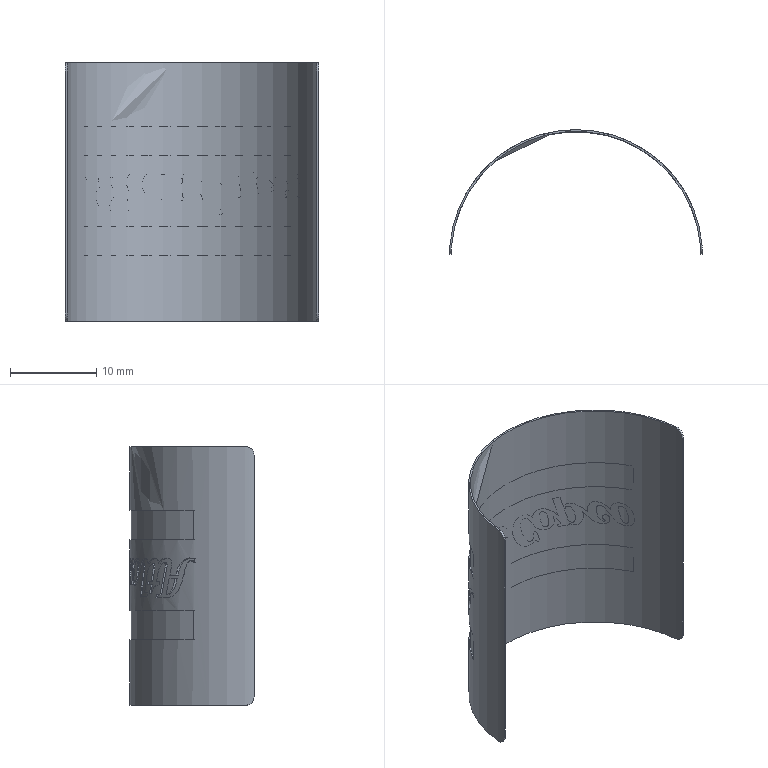Part | STEP file | ASND-0110-4216235500_SPEC | 1 solid | 170 faces | box 29.395 x 14.422 x 30 mm | volume 229.451 mm3 | spline 100 | plane 55 | cylinder 15 | commonest cylinder face diameters 29.4 x6 2 x4 29.1 x4 29 x1